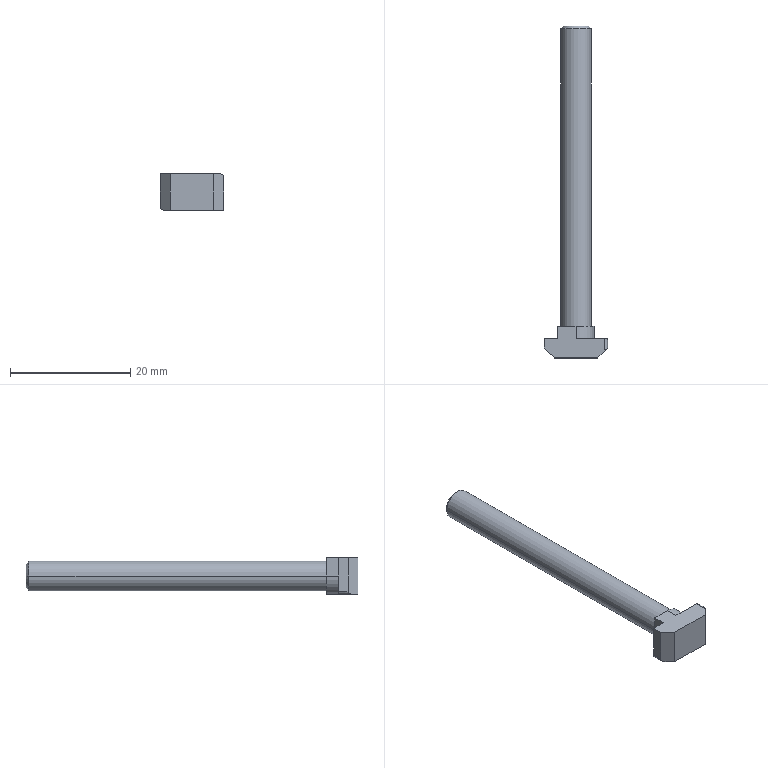Part | SolidWorks | features Fillet 2, ICE 2, Chamfer 1, Extrusion 1, Revolution 1 | 1 solid | 21 faces | box 10.5 x 55.3 x 6 mm | volume 1236 mm3 | plane 13 | cylinder 6 | cone 2 | commonest cylinder face diameters 1 x2 5 x2 6 x2
STEP:
#1=CARTESIAN_POINT('',(-2.009,52.,0.));
#2=VERTEX_POINT('',#1);
#3=CARTESIAN_POINT('',(2.009,52.,0.));
#4=VERTEX_POINT('',#3);
#5=CARTESIAN_POINT('',(0.,52.,0.));
#6=DIRECTION('',(0.,1.,0.));
#7=DIRECTION('',(-1.,0.,0.));
#8=AXIS2_PLACEMENT_3D('',#5,#6,#7);
#9=CIRCLE('',#8,2.009);
#10=EDGE_CURVE('',#2,#4,#9,.T.);
#11=ORIENTED_EDGE('',*,*,#10,.F.);
#12=CARTESIAN_POINT('',(-2.5,51.51,0.));
#13=VERTEX_POINT('',#12);
#14=CARTESIAN_POINT('',(-2.009,52.,0.));
#15=DIRECTION('',(-0.7071,-0.7071,0.));
#16=VECTOR('',#15,1000.);
#17=LINE('',#14,#16);
#18=EDGE_CURVE('',#2,#13,#17,.T.);
#19=ORIENTED_EDGE('',*,*,#18,.T.);
#20=CARTESIAN_POINT('',(2.5,51.51,0.));
#21=VERTEX_POINT('',#20);
#22=CARTESIAN_POINT('',(0.,51.51,0.));
#23=DIRECTION('',(0.,-1.,0.));
#24=DIRECTION('',(-1.,0.,0.));
#25=AXIS2_PLACEMENT_3D('',#22,#23,#24);
#26=CIRCLE('',#25,2.5);
#27=EDGE_CURVE('',#21,#13,#26,.T.);
#28=ORIENTED_EDGE('',*,*,#27,.F.);
#29=CARTESIAN_POINT('',(2.009,52.,0.));
#30=DIRECTION('',(0.7071,-0.7071,0.));
#31=VECTOR('',#30,1000.);
#32=LINE('',#29,#31);
#33=EDGE_CURVE('',#4,#21,#32,.T.);
#34=ORIENTED_EDGE('',*,*,#33,.F.);
#35=EDGE_LOOP('',(#11,#19,#28,#34));
#36=FACE_OUTER_BOUND('',#35,.T.);
#37=CARTESIAN_POINT('',(0.,52.,0.));
#38=DIRECTION('',(0.,-1.,0.));
#39=DIRECTION('',(1.,0.,0.));
#40=AXIS2_PLACEMENT_3D('',#37,#38,#39);
#41=CONICAL_SURFACE('',#40,2.009,0.7854);
#42=ADVANCED_FACE('',(#36),#41,.T.);
#43=CARTESIAN_POINT('',(-2.5,2.,0.));
#44=VERTEX_POINT('',#43);
#45=CARTESIAN_POINT('',(2.5,2.,0.));
#46=VERTEX_POINT('',#45);
#47=CARTESIAN_POINT('',(0.,2.,0.));
#48=DIRECTION('',(0.,1.,0.));
#49=DIRECTION('',(-1.,0.,0.));
#50=AXIS2_PLACEMENT_3D('',#47,#48,#49);
#51=CIRCLE('',#50,2.5);
#52=EDGE_CURVE('',#44,#46,#51,.T.);
#53=ORIENTED_EDGE('',*,*,#52,.T.);
#54=CARTESIAN_POINT('',(2.5,2.,0.));
#55=DIRECTION('',(0.,1.,0.));
#56=VECTOR('',#55,1000.);
#57=LINE('',#54,#56);
#58=EDGE_CURVE('',#46,#21,#57,.T.);
#59=ORIENTED_EDGE('',*,*,#58,.T.);
#60=ORIENTED_EDGE('',*,*,#27,.T.);
#61=CARTESIAN_POINT('',(-2.5,2.,0.));
#62=DIRECTION('',(0.,1.,0.));
#63=VECTOR('',#62,1000.);
#64=LINE('',#61,#63);
#65=EDGE_CURVE('',#44,#13,#64,.T.);
#66=ORIENTED_EDGE('',*,*,#65,.F.);
#67=EDGE_LOOP('',(#53,#59,#60,#66));
#68=FACE_OUTER_BOUND('',#67,.T.);
#69=CARTESIAN_POINT('',(0.,2.,0.));
#70=DIRECTION('',(0.,1.,0.));
#71=DIRECTION('',(-1.,0.,0.));
#72=AXIS2_PLACEMENT_3D('',#69,#70,#71);
#73=CYLINDRICAL_SURFACE('',#72,2.5);
#74=ADVANCED_FACE('',(#68),#73,.T.);
#75=CARTESIAN_POINT('',(-5.25,0.,-2.5));
#76=VERTEX_POINT('',#75);
#77=CARTESIAN_POINT('',(-5.25,0.,3.));
#78=VERTEX_POINT('',#77);
#79=CARTESIAN_POINT('',(-5.25,0.,-3.));
#80=DIRECTION('',(0.,0.,1.));
#81=VECTOR('',#80,1000.);
#82=LINE('',#79,#81);
#83=EDGE_CURVE('',#76,#78,#82,.T.);
#84=ORIENTED_EDGE('',*,*,#83,.F.);
#85=CARTESIAN_POINT('',(-5.25,-1.65,-2.5));
#86=VERTEX_POINT('',#85);
#87=CARTESIAN_POINT('',(-5.25,-1.65,-2.5));
#88=DIRECTION('',(0.,-1.,0.));
#89=VECTOR('',#88,1000.);
#90=LINE('',#87,#89);
#91=EDGE_CURVE('',#76,#86,#90,.T.);
#92=ORIENTED_EDGE('',*,*,#91,.T.);
#93=CARTESIAN_POINT('',(-5.25,-1.65,3.));
#94=VERTEX_POINT('',#93);
#95=CARTESIAN_POINT('',(-5.25,-1.65,3.));
#96=DIRECTION('',(0.,0.,-1.));
#97=VECTOR('',#96,1000.);
#98=LINE('',#95,#97);
#99=EDGE_CURVE('',#94,#86,#98,.T.);
#100=ORIENTED_EDGE('',*,*,#99,.F.);
#101=CARTESIAN_POINT('',(-5.25,-1.65,3.));
#102=DIRECTION('',(0.,1.,0.));
#103=VECTOR('',#102,1000.);
#104=LINE('',#101,#103);
#105=EDGE_CURVE('',#94,#78,#104,.T.);
#106=ORIENTED_EDGE('',*,*,#105,.T.);
#107=EDGE_LOOP('',(#84,#92,#100,#106));
#108=FACE_OUTER_BOUND('',#107,.T.);
#109=CARTESIAN_POINT('',(-5.25,-1.65,3.));
#110=DIRECTION('',(-1.,0.,0.));
#111=DIRECTION('',(0.,-1.,0.));
#112=AXIS2_PLACEMENT_3D('',#109,#110,#111);
#113=PLANE('',#112);
#114=ADVANCED_FACE('',(#108),#113,.T.);
#115=ORIENTED_EDGE('',*,*,#99,.T.);
#116=CARTESIAN_POINT('',(-4.75,-2.15,-3.));
#117=VERTEX_POINT('',#116);
#118=CARTESIAN_POINT('',(-5.25,-1.65,-2.5));
#119=CARTESIAN_POINT('',(-5.25,-1.65,-2.793));
#120=CARTESIAN_POINT('',(-5.043,-1.857,-3.));
#121=CARTESIAN_POINT('',(-4.75,-2.15,-3.));
#122=(BOUNDED_CURVE()B_SPLINE_CURVE(3,(#118,#119,#120,#121),.UNSPECIFIED.,.F.,.F.)B_SPLINE_CURVE_WITH_KNOTS((4,4),(0.,1.571),.UNSPECIFIED.)CURVE()GEOMETRIC_REPRESENTATION_ITEM()RATIONAL_B_SPLINE_CURVE((1.,0.8047,0.8047,1.))REPRESENTATION_ITEM(''));
#123=EDGE_CURVE('',#86,#117,#122,.T.);
#124=ORIENTED_EDGE('',*,*,#123,.T.);
#125=CARTESIAN_POINT('',(-3.6,-3.3,-3.));
#126=VERTEX_POINT('',#125);
#127=CARTESIAN_POINT('',(-3.6,-3.3,-3.));
#128=DIRECTION('',(-0.7071,0.7071,0.));
#129=VECTOR('',#128,1000.);
#130=LINE('',#127,#129);
#131=EDGE_CURVE('',#126,#117,#130,.T.);
#132=ORIENTED_EDGE('',*,*,#131,.F.);
#133=CARTESIAN_POINT('',(-3.6,-3.3,3.));
#134=VERTEX_POINT('',#133);
#135=CARTESIAN_POINT('',(-3.6,-3.3,3.));
#136=DIRECTION('',(0.,0.,-1.));
#137=VECTOR('',#136,1000.);
#138=LINE('',#135,#137);
#139=EDGE_CURVE('',#134,#126,#138,.T.);
#140=ORIENTED_EDGE('',*,*,#139,.F.);
#141=CARTESIAN_POINT('',(-3.6,-3.3,3.));
#142=DIRECTION('',(-0.7071,0.7071,0.));
#143=VECTOR('',#142,1000.);
#144=LINE('',#141,#143);
#145=EDGE_CURVE('',#134,#94,#144,.T.);
#146=ORIENTED_EDGE('',*,*,#145,.T.);
#147=EDGE_LOOP('',(#115,#124,#132,#140,#146));
#148=FACE_OUTER_BOUND('',#147,.T.);
#149=CARTESIAN_POINT('',(-3.6,-3.3,3.));
#150=DIRECTION('',(-0.7071,-0.7071,0.));
#151=DIRECTION('',(0.7071,-0.7071,0.));
#152=AXIS2_PLACEMENT_3D('',#149,#150,#151);
#153=PLANE('',#152);
#154=ADVANCED_FACE('',(#148),#153,.T.);
#155=CARTESIAN_POINT('',(3.6,-3.3,-3.));
#156=VERTEX_POINT('',#155);
#157=CARTESIAN_POINT('',(3.6,-3.3,-3.));
#158=DIRECTION('',(-1.,0.,0.));
#159=VECTOR('',#158,1000.);
#160=LINE('',#157,#159);
#161=EDGE_CURVE('',#156,#126,#160,.T.);
#162=ORIENTED_EDGE('',*,*,#161,.F.);
#163=CARTESIAN_POINT('',(3.6,-3.3,3.));
#164=VERTEX_POINT('',#163);
#165=CARTESIAN_POINT('',(3.6,-3.3,3.));
#166=DIRECTION('',(0.,0.,-1.));
#167=VECTOR('',#166,1000.);
#168=LINE('',#165,#167);
#169=EDGE_CURVE('',#164,#156,#168,.T.);
#170=ORIENTED_EDGE('',*,*,#169,.F.);
#171=CARTESIAN_POINT('',(3.6,-3.3,3.));
#172=DIRECTION('',(-1.,0.,0.));
#173=VECTOR('',#172,1000.);
#174=LINE('',#171,#173);
#175=EDGE_CURVE('',#164,#134,#174,.T.);
#176=ORIENTED_EDGE('',*,*,#175,.T.);
#177=ORIENTED_EDGE('',*,*,#139,.T.);
#178=EDGE_LOOP('',(#162,#170,#176,#177));
#179=FACE_OUTER_BOUND('',#178,.T.);
#180=CARTESIAN_POINT('',(3.6,-3.3,3.));
#181=DIRECTION('',(0.,-1.,0.));
#182=DIRECTION('',(0.,0.,-1.));
#183=AXIS2_PLACEMENT_3D('',#180,#181,#182);
#184=PLANE('',#183);
#185=ADVANCED_FACE('',(#179),#184,.T.);
#186=CARTESIAN_POINT('',(5.25,-1.65,2.5));
#187=VERTEX_POINT('',#186);
#188=CARTESIAN_POINT('',(5.25,-1.65,-3.));
#189=VERTEX_POINT('',#188);
#190=CARTESIAN_POINT('',(5.25,-1.65,3.));
#191=DIRECTION('',(0.,0.,-1.));
#192=VECTOR('',#191,1000.);
#193=LINE('',#190,#192);
#194=EDGE_CURVE('',#187,#189,#193,.T.);
#195=ORIENTED_EDGE('',*,*,#194,.F.);
#196=CARTESIAN_POINT('',(4.75,-2.15,3.));
#197=VERTEX_POINT('',#196);
#198=CARTESIAN_POINT('',(5.25,-1.65,2.5));
#199=CARTESIAN_POINT('',(5.25,-1.65,2.793));
#200=CARTESIAN_POINT('',(5.043,-1.857,3.));
#201=CARTESIAN_POINT('',(4.75,-2.15,3.));
#202=(BOUNDED_CURVE()B_SPLINE_CURVE(3,(#198,#199,#200,#201),.UNSPECIFIED.,.F.,.F.)B_SPLINE_CURVE_WITH_KNOTS((4,4),(0.,1.571),.UNSPECIFIED.)CURVE()GEOMETRIC_REPRESENTATION_ITEM()RATIONAL_B_SPLINE_CURVE((1.,0.8047,0.8047,1.))REPRESENTATION_ITEM(''));
#203=EDGE_CURVE('',#187,#197,#202,.T.);
#204=ORIENTED_EDGE('',*,*,#203,.T.);
#205=CARTESIAN_POINT('',(5.25,-1.65,3.));
#206=DIRECTION('',(-0.7071,-0.7071,0.));
#207=VECTOR('',#206,1000.);
#208=LINE('',#205,#207);
#209=EDGE_CURVE('',#197,#164,#208,.T.);
#210=ORIENTED_EDGE('',*,*,#209,.T.);
#211=ORIENTED_EDGE('',*,*,#169,.T.);
#212=CARTESIAN_POINT('',(5.25,-1.65,-3.));
#213=DIRECTION('',(-0.7071,-0.7071,0.));
#214=VECTOR('',#213,1000.);
#215=LINE('',#212,#214);
#216=EDGE_CURVE('',#189,#156,#215,.T.);
#217=ORIENTED_EDGE('',*,*,#216,.F.);
#218=EDGE_LOOP('',(#195,#204,#210,#211,#217));
#219=FACE_OUTER_BOUND('',#218,.T.);
#220=CARTESIAN_POINT('',(5.25,-1.65,3.));
#221=DIRECTION('',(0.7071,-0.7071,0.));
#222=DIRECTION('',(0.7071,0.7071,0.));
#223=AXIS2_PLACEMENT_3D('',#220,#221,#222);
#224=PLANE('',#223);
#225=ADVANCED_FACE('',(#219),#224,.T.);
#226=CARTESIAN_POINT('',(5.25,0.,-3.));
#227=VERTEX_POINT('',#226);
#228=CARTESIAN_POINT('',(5.25,0.,2.5));
#229=VERTEX_POINT('',#228);
#230=CARTESIAN_POINT('',(5.25,0.,-3.));
#231=DIRECTION('',(0.,0.,1.));
#232=VECTOR('',#231,1000.);
#233=LINE('',#230,#232);
#234=EDGE_CURVE('',#227,#229,#233,.T.);
#235=ORIENTED_EDGE('',*,*,#234,.T.);
#236=CARTESIAN_POINT('',(5.25,-1.65,2.5));
#237=DIRECTION('',(0.,-1.,0.));
#238=VECTOR('',#237,1000.);
#239=LINE('',#236,#238);
#240=EDGE_CURVE('',#229,#187,#239,.T.);
#241=ORIENTED_EDGE('',*,*,#240,.T.);
#242=ORIENTED_EDGE('',*,*,#194,.T.);
#243=CARTESIAN_POINT('',(5.25,2.,-3.));
#244=DIRECTION('',(0.,-1.,0.));
#245=VECTOR('',#244,1000.);
#246=LINE('',#243,#245);
#247=EDGE_CURVE('',#227,#189,#246,.T.);
#248=ORIENTED_EDGE('',*,*,#247,.F.);
#249=EDGE_LOOP('',(#235,#241,#242,#248));
#250=FACE_OUTER_BOUND('',#249,.T.);
#251=CARTESIAN_POINT('',(5.25,2.,3.));
#252=DIRECTION('',(1.,0.,0.));
#253=DIRECTION('',(0.,0.,-1.));
#254=AXIS2_PLACEMENT_3D('',#251,#252,#253);
#255=PLANE('',#254);
#256=ADVANCED_FACE('',(#250),#255,.T.);
#257=ORIENTED_EDGE('',*,*,#52,.F.);
#258=CARTESIAN_POINT('',(0.,2.,0.));
#259=DIRECTION('',(0.,1.,0.));
#260=DIRECTION('',(-1.,0.,0.));
#261=AXIS2_PLACEMENT_3D('',#258,#259,#260);
#262=CIRCLE('',#261,2.5);
#263=EDGE_CURVE('',#46,#44,#262,.T.);
#264=ORIENTED_EDGE('',*,*,#263,.F.);
#265=EDGE_LOOP('',(#257,#264));
#266=FACE_BOUND('',#265,.T.);
#267=CARTESIAN_POINT('',(-3.,2.,3.));
#268=VERTEX_POINT('',#267);
#269=CARTESIAN_POINT('',(0.,2.,3.));
#270=VERTEX_POINT('',#269);
#271=CARTESIAN_POINT('',(-5.25,2.,3.));
#272=DIRECTION('',(1.,0.,0.));
#273=VECTOR('',#272,1000.);
#274=LINE('',#271,#273);
#275=EDGE_CURVE('',#268,#270,#274,.T.);
#276=ORIENTED_EDGE('',*,*,#275,.T.);
#277=CARTESIAN_POINT('',(3.,2.,0.));
#278=VERTEX_POINT('',#277);
#279=CARTESIAN_POINT('',(0.,2.,0.));
#280=DIRECTION('',(0.,1.,0.));
#281=DIRECTION('',(0.,0.,1.));
#282=AXIS2_PLACEMENT_3D('',#279,#280,#281);
#283=CIRCLE('',#282,3.);
#284=EDGE_CURVE('',#270,#278,#283,.T.);
#285=ORIENTED_EDGE('',*,*,#284,.T.);
#286=CARTESIAN_POINT('',(3.,2.,-3.));
#287=VERTEX_POINT('',#286);
#288=CARTESIAN_POINT('',(3.,2.,-3.));
#289=DIRECTION('',(0.,0.,1.));
#290=VECTOR('',#289,1000.);
#291=LINE('',#288,#290);
#292=EDGE_CURVE('',#287,#278,#291,.T.);
#293=ORIENTED_EDGE('',*,*,#292,.F.);
#294=CARTESIAN_POINT('',(0.,2.,-3.));
#295=VERTEX_POINT('',#294);
#296=CARTESIAN_POINT('',(-5.25,2.,-3.));
#297=DIRECTION('',(1.,0.,0.));
#298=VECTOR('',#297,1000.);
#299=LINE('',#296,#298);
#300=EDGE_CURVE('',#295,#287,#299,.T.);
#301=ORIENTED_EDGE('',*,*,#300,.F.);
#302=CARTESIAN_POINT('',(-3.,2.,0.));
#303=VERTEX_POINT('',#302);
#304=CARTESIAN_POINT('',(0.,2.,0.));
#305=DIRECTION('',(0.,1.,0.));
#306=DIRECTION('',(0.,0.,1.));
#307=AXIS2_PLACEMENT_3D('',#304,#305,#306);
#308=CIRCLE('',#307,3.);
#309=EDGE_CURVE('',#295,#303,#308,.T.);
#310=ORIENTED_EDGE('',*,*,#309,.T.);
#311=CARTESIAN_POINT('',(-3.,2.,-3.));
#312=DIRECTION('',(0.,0.,1.));
#313=VECTOR('',#312,1000.);
#314=LINE('',#311,#313);
#315=EDGE_CURVE('',#303,#268,#314,.T.);
#316=ORIENTED_EDGE('',*,*,#315,.T.);
#317=EDGE_LOOP('',(#276,#285,#293,#301,#310,#316));
#318=FACE_OUTER_BOUND('',#317,.T.);
#319=CARTESIAN_POINT('',(-5.25,2.,3.));
#320=DIRECTION('',(0.,1.,0.));
#321=DIRECTION('',(0.,0.,1.));
#322=AXIS2_PLACEMENT_3D('',#319,#320,#321);
#323=PLANE('',#322);
#324=ADVANCED_FACE('',(#266,#318),#323,.T.);
#325=CARTESIAN_POINT('',(0.,0.,3.));
#326=VERTEX_POINT('',#325);
#327=CARTESIAN_POINT('',(4.75,0.,3.));
#328=VERTEX_POINT('',#327);
#329=CARTESIAN_POINT('',(3.,0.,3.));
#330=DIRECTION('',(1.,0.,0.));
#331=VECTOR('',#330,1000.);
#332=LINE('',#329,#331);
#333=EDGE_CURVE('',#326,#328,#332,.T.);
#334=ORIENTED_EDGE('',*,*,#333,.F.);
#335=CARTESIAN_POINT('',(0.,0.,3.));
#336=DIRECTION('',(0.,1.,0.));
#337=VECTOR('',#336,1000.);
#338=LINE('',#335,#337);
#339=EDGE_CURVE('',#326,#270,#338,.T.);
#340=ORIENTED_EDGE('',*,*,#339,.T.);
#341=ORIENTED_EDGE('',*,*,#275,.F.);
#342=CARTESIAN_POINT('',(-3.,0.,3.));
#343=VERTEX_POINT('',#342);
#344=CARTESIAN_POINT('',(-3.,0.,3.));
#345=DIRECTION('',(0.,1.,0.));
#346=VECTOR('',#345,1000.);
#347=LINE('',#344,#346);
#348=EDGE_CURVE('',#343,#268,#347,.T.);
#349=ORIENTED_EDGE('',*,*,#348,.F.);
#350=CARTESIAN_POINT('',(-5.25,0.,3.));
#351=DIRECTION('',(1.,0.,0.));
#352=VECTOR('',#351,1000.);
#353=LINE('',#350,#352);
#354=EDGE_CURVE('',#78,#343,#353,.T.);
#355=ORIENTED_EDGE('',*,*,#354,.F.);
#356=ORIENTED_EDGE('',*,*,#105,.F.);
#357=ORIENTED_EDGE('',*,*,#145,.F.);
#358=ORIENTED_EDGE('',*,*,#175,.F.);
#359=ORIENTED_EDGE('',*,*,#209,.F.);
#360=CARTESIAN_POINT('',(4.75,0.,3.));
#361=DIRECTION('',(0.,1.,0.));
#362=VECTOR('',#361,1000.);
#363=LINE('',#360,#362);
#364=EDGE_CURVE('',#197,#328,#363,.T.);
#365=ORIENTED_EDGE('',*,*,#364,.T.);
#366=EDGE_LOOP('',(#334,#340,#341,#349,#355,#356,#357,#358,#359,#365));
#367=FACE_OUTER_BOUND('',#366,.T.);
#368=CARTESIAN_POINT('',(0.,0.,3.));
#369=DIRECTION('',(0.,0.,-1.));
#370=DIRECTION('',(-1.,0.,0.));
#371=AXIS2_PLACEMENT_3D('',#368,#369,#370);
#372=PLANE('',#371);
#373=ADVANCED_FACE('',(#367),#372,.F.);
#374=CARTESIAN_POINT('',(-4.75,0.,-3.));
#375=VERTEX_POINT('',#374);
#376=CARTESIAN_POINT('',(0.,0.,-3.));
#377=VERTEX_POINT('',#376);
#378=CARTESIAN_POINT('',(-5.25,0.,-3.));
#379=DIRECTION('',(1.,0.,0.));
#380=VECTOR('',#379,1000.);
#381=LINE('',#378,#380);
#382=EDGE_CURVE('',#375,#377,#381,.T.);
#383=ORIENTED_EDGE('',*,*,#382,.T.);
#384=CARTESIAN_POINT('',(0.,2.,-3.));
#385=DIRECTION('',(0.,1.,0.));
#386=VECTOR('',#385,1000.);
#387=LINE('',#384,#386);
#388=EDGE_CURVE('',#377,#295,#387,.T.);
#389=ORIENTED_EDGE('',*,*,#388,.T.);
#390=ORIENTED_EDGE('',*,*,#300,.T.);
#391=CARTESIAN_POINT('',(3.,0.,-3.));
#392=VERTEX_POINT('',#391);
#393=CARTESIAN_POINT('',(3.,2.,-3.));
#394=DIRECTION('',(0.,-1.,0.));
#395=VECTOR('',#394,1000.);
#396=LINE('',#393,#395);
#397=EDGE_CURVE('',#287,#392,#396,.T.);
#398=ORIENTED_EDGE('',*,*,#397,.T.);
#399=CARTESIAN_POINT('',(3.,0.,-3.));
#400=DIRECTION('',(1.,0.,0.));
#401=VECTOR('',#400,1000.);
#402=LINE('',#399,#401);
#403=EDGE_CURVE('',#392,#227,#402,.T.);
#404=ORIENTED_EDGE('',*,*,#403,.T.);
#405=ORIENTED_EDGE('',*,*,#247,.T.);
#406=ORIENTED_EDGE('',*,*,#216,.T.);
#407=ORIENTED_EDGE('',*,*,#161,.T.);
#408=ORIENTED_EDGE('',*,*,#131,.T.);
#409=CARTESIAN_POINT('',(-4.75,0.,-3.));
#410=DIRECTION('',(0.,1.,0.));
#411=VECTOR('',#410,1000.);
#412=LINE('',#409,#411);
#413=EDGE_CURVE('',#117,#375,#412,.T.);
#414=ORIENTED_EDGE('',*,*,#413,.T.);
#415=EDGE_LOOP('',(#383,#389,#390,#398,#404,#405,#406,#407,#408,#414));
#416=FACE_OUTER_BOUND('',#415,.T.);
#417=CARTESIAN_POINT('',(0.,0.,-3.));
#418=DIRECTION('',(0.,0.,-1.));
#419=DIRECTION('',(-1.,0.,0.));
#420=AXIS2_PLACEMENT_3D('',#417,#418,#419);
#421=PLANE('',#420);
#422=ADVANCED_FACE('',(#416),#421,.T.);
#423=ORIENTED_EDGE('',*,*,#315,.F.);
#424=CARTESIAN_POINT('',(-3.,0.,0.));
#425=VERTEX_POINT('',#424);
#426=CARTESIAN_POINT('',(-3.,0.,0.));
#427=DIRECTION('',(0.,-1.,0.));
#428=VECTOR('',#427,1000.);
#429=LINE('',#426,#428);
#430=EDGE_CURVE('',#303,#425,#429,.T.);
#431=ORIENTED_EDGE('',*,*,#430,.T.);
#432=CARTESIAN_POINT('',(-3.,0.,-3.));
#433=DIRECTION('',(0.,0.,1.));
#434=VECTOR('',#433,1000.);
#435=LINE('',#432,#434);
#436=EDGE_CURVE('',#425,#343,#435,.T.);
#437=ORIENTED_EDGE('',*,*,#436,.T.);
#438=ORIENTED_EDGE('',*,*,#348,.T.);
#439=EDGE_LOOP('',(#423,#431,#437,#438));
#440=FACE_OUTER_BOUND('',#439,.T.);
#441=CARTESIAN_POINT('',(-3.,0.,-3.));
#442=DIRECTION('',(1.,0.,0.));
#443=DIRECTION('',(0.,0.,-1.));
#444=AXIS2_PLACEMENT_3D('',#441,#442,#443);
#445=PLANE('',#444);
#446=ADVANCED_FACE('',(#440),#445,.F.);
#447=ORIENTED_EDGE('',*,*,#382,.F.);
#448=CARTESIAN_POINT('',(-4.75,0.,-2.5));
#449=DIRECTION('',(0.,1.,0.));
#450=DIRECTION('',(0.,0.,-1.));
#451=AXIS2_PLACEMENT_3D('',#448,#449,#450);
#452=CIRCLE('',#451,0.5);
#453=EDGE_CURVE('',#375,#76,#452,.T.);
#454=ORIENTED_EDGE('',*,*,#453,.T.);
#455=ORIENTED_EDGE('',*,*,#83,.T.);
#456=ORIENTED_EDGE('',*,*,#354,.T.);
#457=ORIENTED_EDGE('',*,*,#436,.F.);
#458=CARTESIAN_POINT('',(0.,0.,0.));
#459=DIRECTION('',(0.,-1.,0.));
#460=DIRECTION('',(0.,0.,-1.));
#461=AXIS2_PLACEMENT_3D('',#458,#459,#460);
#462=CIRCLE('',#461,3.);
#463=EDGE_CURVE('',#425,#377,#462,.T.);
#464=ORIENTED_EDGE('',*,*,#463,.T.);
#465=EDGE_LOOP('',(#447,#454,#455,#456,#457,#464));
#466=FACE_OUTER_BOUND('',#465,.T.);
#467=CARTESIAN_POINT('',(-5.25,0.,-3.));
#468=DIRECTION('',(0.,-1.,0.));
#469=DIRECTION('',(0.,0.,-1.));
#470=AXIS2_PLACEMENT_3D('',#467,#468,#469);
#471=PLANE('',#470);
#472=ADVANCED_FACE('',(#466),#471,.F.);
#473=ORIENTED_EDGE('',*,*,#292,.T.);
#474=CARTESIAN_POINT('',(3.,0.,0.));
#475=VERTEX_POINT('',#474);
#476=CARTESIAN_POINT('',(3.,2.,0.));
#477=DIRECTION('',(0.,-1.,0.));
#478=VECTOR('',#477,1000.);
#479=LINE('',#476,#478);
#480=EDGE_CURVE('',#278,#475,#479,.T.);
#481=ORIENTED_EDGE('',*,*,#480,.T.);
#482=CARTESIAN_POINT('',(3.,0.,-3.));
#483=DIRECTION('',(0.,0.,1.));
#484=VECTOR('',#483,1000.);
#485=LINE('',#482,#484);
#486=EDGE_CURVE('',#392,#475,#485,.T.);
#487=ORIENTED_EDGE('',*,*,#486,.F.);
#488=ORIENTED_EDGE('',*,*,#397,.F.);
#489=EDGE_LOOP('',(#473,#481,#487,#488));
#490=FACE_OUTER_BOUND('',#489,.T.);
#491=CARTESIAN_POINT('',(3.,2.,-3.));
#492=DIRECTION('',(-1.,0.,0.));
#493=DIRECTION('',(0.,0.,1.));
#494=AXIS2_PLACEMENT_3D('',#491,#492,#493);
#495=PLANE('',#494);
#496=ADVANCED_FACE('',(#490),#495,.F.);
#497=ORIENTED_EDGE('',*,*,#333,.T.);
#498=CARTESIAN_POINT('',(4.75,0.,2.5));
#499=DIRECTION('',(0.,1.,0.));
#500=DIRECTION('',(0.,0.,-1.));
#501=AXIS2_PLACEMENT_3D('',#498,#499,#500);
#502=CIRCLE('',#501,0.5);
#503=EDGE_CURVE('',#328,#229,#502,.T.);
#504=ORIENTED_EDGE('',*,*,#503,.T.);
#505=ORIENTED_EDGE('',*,*,#234,.F.);
#506=ORIENTED_EDGE('',*,*,#403,.F.);
#507=ORIENTED_EDGE('',*,*,#486,.T.);
#508=CARTESIAN_POINT('',(0.,0.,0.));
#509=DIRECTION('',(0.,-1.,0.));
#510=DIRECTION('',(0.,0.,-1.));
#511=AXIS2_PLACEMENT_3D('',#508,#509,#510);
#512=CIRCLE('',#511,3.);
#513=EDGE_CURVE('',#475,#326,#512,.T.);
#514=ORIENTED_EDGE('',*,*,#513,.T.);
#515=EDGE_LOOP('',(#497,#504,#505,#506,#507,#514));
#516=FACE_OUTER_BOUND('',#515,.T.);
#517=CARTESIAN_POINT('',(3.,0.,-3.));
#518=DIRECTION('',(0.,-1.,0.));
#519=DIRECTION('',(0.,0.,-1.));
#520=AXIS2_PLACEMENT_3D('',#517,#518,#519);
#521=PLANE('',#520);
#522=ADVANCED_FACE('',(#516),#521,.F.);
#523=ORIENTED_EDGE('',*,*,#58,.F.);
#524=ORIENTED_EDGE('',*,*,#263,.T.);
#525=ORIENTED_EDGE('',*,*,#65,.T.);
#526=CARTESIAN_POINT('',(0.,51.51,0.));
#527=DIRECTION('',(0.,-1.,0.));
#528=DIRECTION('',(-1.,0.,0.));
#529=AXIS2_PLACEMENT_3D('',#526,#527,#528);
#530=CIRCLE('',#529,2.5);
#531=EDGE_CURVE('',#13,#21,#530,.T.);
#532=ORIENTED_EDGE('',*,*,#531,.T.);
#533=EDGE_LOOP('',(#523,#524,#525,#532));
#534=FACE_OUTER_BOUND('',#533,.T.);
#535=CARTESIAN_POINT('',(0.,2.,0.));
#536=DIRECTION('',(0.,1.,0.));
#537=DIRECTION('',(-1.,0.,0.));
#538=AXIS2_PLACEMENT_3D('',#535,#536,#537);
#539=CYLINDRICAL_SURFACE('',#538,2.5);
#540=ADVANCED_FACE('',(#534),#539,.T.);
#541=CARTESIAN_POINT('',(0.,52.,0.));
#542=DIRECTION('',(0.,1.,0.));
#543=DIRECTION('',(-1.,0.,0.));
#544=AXIS2_PLACEMENT_3D('',#541,#542,#543);
#545=CIRCLE('',#544,2.009);
#546=EDGE_CURVE('',#4,#2,#545,.T.);
#547=ORIENTED_EDGE('',*,*,#546,.T.);
#548=ORIENTED_EDGE('',*,*,#10,.T.);
#549=EDGE_LOOP('',(#547,#548));
#550=FACE_OUTER_BOUND('',#549,.T.);
#551=CARTESIAN_POINT('',(0.,52.,0.));
#552=DIRECTION('',(0.,1.,0.));
#553=DIRECTION('',(-1.,0.,0.));
#554=AXIS2_PLACEMENT_3D('',#551,#552,#553);
#555=PLANE('',#554);
#556=ADVANCED_FACE('',(#550),#555,.T.);
#557=ORIENTED_EDGE('',*,*,#18,.F.);
#558=ORIENTED_EDGE('',*,*,#546,.F.);
#559=ORIENTED_EDGE('',*,*,#33,.T.);
#560=ORIENTED_EDGE('',*,*,#531,.F.);
#561=EDGE_LOOP('',(#557,#558,#559,#560));
#562=FACE_OUTER_BOUND('',#561,.T.);
#563=CARTESIAN_POINT('',(0.,52.,0.));
#564=DIRECTION('',(0.,-1.,0.));
#565=DIRECTION('',(1.,0.,0.));
#566=AXIS2_PLACEMENT_3D('',#563,#564,#565);
#567=CONICAL_SURFACE('',#566,2.009,0.7854);
#568=ADVANCED_FACE('',(#562),#567,.T.);
#569=ORIENTED_EDGE('',*,*,#123,.F.);
#570=ORIENTED_EDGE('',*,*,#91,.F.);
#571=ORIENTED_EDGE('',*,*,#453,.F.);
#572=ORIENTED_EDGE('',*,*,#413,.F.);
#573=EDGE_LOOP('',(#569,#570,#571,#572));
#574=FACE_OUTER_BOUND('',#573,.T.);
#575=CARTESIAN_POINT('',(-4.75,0.,-2.5));
#576=DIRECTION('',(0.,1.,0.));
#577=DIRECTION('',(-1.,0.,0.));
#578=AXIS2_PLACEMENT_3D('',#575,#576,#577);
#579=CYLINDRICAL_SURFACE('',#578,0.5);
#580=ADVANCED_FACE('',(#574),#579,.T.);
#581=ORIENTED_EDGE('',*,*,#503,.F.);
#582=ORIENTED_EDGE('',*,*,#364,.F.);
#583=ORIENTED_EDGE('',*,*,#203,.F.);
#584=ORIENTED_EDGE('',*,*,#240,.F.);
#585=EDGE_LOOP('',(#581,#582,#583,#584));
#586=FACE_OUTER_BOUND('',#585,.T.);
#587=CARTESIAN_POINT('',(4.75,2.,2.5));
#588=DIRECTION('',(0.,1.,0.));
#589=DIRECTION('',(0.,0.,1.));
#590=AXIS2_PLACEMENT_3D('',#587,#588,#589);
#591=CYLINDRICAL_SURFACE('',#590,0.5);
#592=ADVANCED_FACE('',(#586),#591,.T.);
#593=ORIENTED_EDGE('',*,*,#284,.F.);
#594=ORIENTED_EDGE('',*,*,#339,.F.);
#595=ORIENTED_EDGE('',*,*,#513,.F.);
#596=ORIENTED_EDGE('',*,*,#480,.F.);
#597=EDGE_LOOP('',(#593,#594,#595,#596));
#598=FACE_OUTER_BOUND('',#597,.T.);
#599=CARTESIAN_POINT('',(0.,2.,0.));
#600=DIRECTION('',(0.,-1.,0.));
#601=DIRECTION('',(0.,0.,-1.));
#602=AXIS2_PLACEMENT_3D('',#599,#600,#601);
#603=CYLINDRICAL_SURFACE('',#602,3.);
#604=ADVANCED_FACE('',(#598),#603,.T.);
#605=ORIENTED_EDGE('',*,*,#463,.F.);
#606=ORIENTED_EDGE('',*,*,#430,.F.);
#607=ORIENTED_EDGE('',*,*,#309,.F.);
#608=ORIENTED_EDGE('',*,*,#388,.F.);
#609=EDGE_LOOP('',(#605,#606,#607,#608));
#610=FACE_OUTER_BOUND('',#609,.T.);
#611=CARTESIAN_POINT('',(0.,0.,0.));
#612=DIRECTION('',(0.,-1.,0.));
#613=DIRECTION('',(0.,0.,-1.));
#614=AXIS2_PLACEMENT_3D('',#611,#612,#613);
#615=CYLINDRICAL_SURFACE('',#614,3.);
#616=ADVANCED_FACE('',(#610),#615,.T.);
#617=CLOSED_SHELL('',(#42,#74,#114,#154,#185,#225,#256,#324,#373,#422,#446,#472,#496,#522,#540,#556,#568,#580,#592,#604,#616));
#618=MANIFOLD_SOLID_BREP('',#617);
#619=CARTESIAN_POINT('',(0.,0.,0.));
#620=DIRECTION('',(0.,0.,1.));
#621=DIRECTION('',(1.,0.,0.));
#622=AXIS2_PLACEMENT_3D('',#619,#620,#621);
#623=(LENGTH_UNIT()NAMED_UNIT(*)SI_UNIT(.MILLI.,.METRE.));
#624=UNCERTAINTY_MEASURE_WITH_UNIT(LENGTH_MEASURE(0.00001),#623,'','');
#625=(NAMED_UNIT(*)PLANE_ANGLE_UNIT()SI_UNIT($,.RADIAN.));
#626=(NAMED_UNIT(*)SI_UNIT($,.STERADIAN.)SOLID_ANGLE_UNIT());
#627=(GEOMETRIC_REPRESENTATION_CONTEXT(3)GLOBAL_UNCERTAINTY_ASSIGNED_CONTEXT((#624))GLOBAL_UNIT_ASSIGNED_CONTEXT((#623,#625,#626))REPRESENTATION_CONTEXT('',''));
#628=ADVANCED_BREP_SHAPE_REPRESENTATION('',(#618,#622),#627);